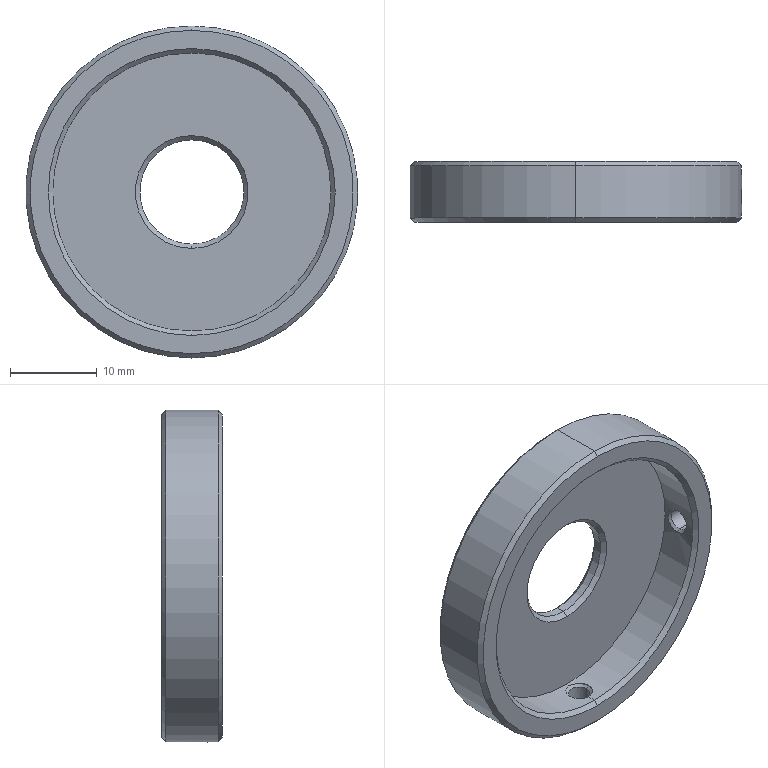Part | SolidWorks | features 3DProfileFeature 1, HoleWzd 1, ICE 1, Revolution 1 | 1 solid | 33 faces | box 38.2 x 7 x 38.2 mm | volume 3692 mm3 | cylinder 16 | cone 14 | plane 3 | commonest cylinder face diameters 3.05 x6 2.5 x4 12 x2 32 x2 38.2 x2
STEP:
#1=CARTESIAN_POINT('',(16.275,3.,-1.25));
#2=VERTEX_POINT('',#1);
#3=CARTESIAN_POINT('',(16.275,3.,1.25));
#4=VERTEX_POINT('',#3);
#5=CARTESIAN_POINT('',(16.275,3.,0.));
#6=DIRECTION('',(-1.,0.,0.));
#7=DIRECTION('',(0.,0.,1.));
#8=AXIS2_PLACEMENT_3D('',#5,#6,#7);
#9=CIRCLE('',#8,1.25);
#10=EDGE_CURVE('',#2,#4,#9,.T.);
#11=ORIENTED_EDGE('',*,*,#10,.F.);
#12=CARTESIAN_POINT('',(16.,3.,-1.525));
#13=VERTEX_POINT('',#12);
#14=CARTESIAN_POINT('',(16.,3.,-1.525));
#15=DIRECTION('',(-0.7071,0.,-0.7071));
#16=VECTOR('',#15,1000.);
#17=LINE('',#14,#16);
#18=EDGE_CURVE('',#2,#13,#17,.T.);
#19=ORIENTED_EDGE('',*,*,#18,.T.);
#20=CARTESIAN_POINT('',(16.,1.475,0.));
#21=VERTEX_POINT('',#20);
#22=CARTESIAN_POINT('',(16.,3.,0.));
#23=DIRECTION('',(-1.,0.,0.));
#24=DIRECTION('',(0.,0.,1.));
#25=AXIS2_PLACEMENT_3D('',#22,#23,#24);
#26=CIRCLE('',#25,1.525);
#27=EDGE_CURVE('',#13,#21,#26,.T.);
#28=ORIENTED_EDGE('',*,*,#27,.T.);
#29=CARTESIAN_POINT('',(16.,3.,1.525));
#30=VERTEX_POINT('',#29);
#31=CARTESIAN_POINT('',(16.,3.,0.));
#32=DIRECTION('',(-1.,0.,0.));
#33=DIRECTION('',(0.,0.,1.));
#34=AXIS2_PLACEMENT_3D('',#31,#32,#33);
#35=CIRCLE('',#34,1.525);
#36=EDGE_CURVE('',#21,#30,#35,.T.);
#37=ORIENTED_EDGE('',*,*,#36,.T.);
#38=CARTESIAN_POINT('',(16.,3.,1.525));
#39=DIRECTION('',(-0.7071,0.,0.7071));
#40=VECTOR('',#39,1000.);
#41=LINE('',#38,#40);
#42=EDGE_CURVE('',#4,#30,#41,.T.);
#43=ORIENTED_EDGE('',*,*,#42,.F.);
#44=EDGE_LOOP('',(#11,#19,#28,#37,#43));
#45=FACE_OUTER_BOUND('',#44,.T.);
#46=CARTESIAN_POINT('',(16.,3.,0.));
#47=DIRECTION('',(-1.,0.,0.));
#48=DIRECTION('',(0.,0.,1.));
#49=AXIS2_PLACEMENT_3D('',#46,#47,#48);
#50=CONICAL_SURFACE('',#49,1.525,0.7854);
#51=ADVANCED_FACE('',(#45),#50,.F.);
#52=CARTESIAN_POINT('',(19.059,3.,1.25));
#53=VERTEX_POINT('',#52);
#54=CARTESIAN_POINT('',(19.059,3.,-1.25));
#55=VERTEX_POINT('',#54);
#56=CARTESIAN_POINT('',(19.059,3.,1.25));
#57=CARTESIAN_POINT('',(19.059,2.835,1.25));
#58=CARTESIAN_POINT('',(19.061,2.673,1.218));
#59=CARTESIAN_POINT('',(19.067,2.446,1.123));
#60=CARTESIAN_POINT('',(19.069,2.374,1.085));
#61=CARTESIAN_POINT('',(19.074,2.238,0.9943));
#62=CARTESIAN_POINT('',(19.077,2.174,0.9415));
#63=CARTESIAN_POINT('',(19.085,2.001,0.7685));
#64=CARTESIAN_POINT('',(19.09,1.908,0.6291));
#65=CARTESIAN_POINT('',(19.098,1.783,0.3284));
#66=CARTESIAN_POINT('',(19.1,1.75,0.1642));
#67=CARTESIAN_POINT('',(19.1,1.75,-0.1661));
#68=CARTESIAN_POINT('',(19.098,1.783,-0.3282));
#69=CARTESIAN_POINT('',(19.09,1.908,-0.6308));
#70=CARTESIAN_POINT('',(19.085,2.001,-0.7694));
#71=CARTESIAN_POINT('',(19.074,2.232,-0.9997));
#72=CARTESIAN_POINT('',(19.069,2.372,-1.093));
#73=CARTESIAN_POINT('',(19.061,2.672,-1.217));
#74=CARTESIAN_POINT('',(19.059,2.837,-1.25));
#75=CARTESIAN_POINT('',(19.059,3.,-1.25));
#76=B_SPLINE_CURVE_WITH_KNOTS('',3,(#56,#57,#58,#59,#60,#61,#62,#63,#64,#65,#66,#67,#68,#69,#70,#71,#72,#73,#74,#75),.UNSPECIFIED.,.F.,.F.,(4,2,2,2,2,2,2,2,2,4),(0.005864,0.006353,0.006597,0.006841,0.00733,0.007818,0.008307,0.008795,0.009284,0.009772),.UNSPECIFIED.);
#77=EDGE_CURVE('',#53,#55,#76,.T.);
#78=ORIENTED_EDGE('',*,*,#77,.T.);
#79=CARTESIAN_POINT('',(16.,3.,-1.25));
#80=DIRECTION('',(-1.,0.,0.));
#81=VECTOR('',#80,1000.);
#82=LINE('',#79,#81);
#83=EDGE_CURVE('',#55,#2,#82,.T.);
#84=ORIENTED_EDGE('',*,*,#83,.T.);
#85=ORIENTED_EDGE('',*,*,#10,.T.);
#86=CARTESIAN_POINT('',(16.,3.,1.25));
#87=DIRECTION('',(-1.,0.,0.));
#88=VECTOR('',#87,1000.);
#89=LINE('',#86,#88);
#90=EDGE_CURVE('',#53,#4,#89,.T.);
#91=ORIENTED_EDGE('',*,*,#90,.F.);
#92=EDGE_LOOP('',(#78,#84,#85,#91));
#93=FACE_OUTER_BOUND('',#92,.T.);
#94=CARTESIAN_POINT('',(16.,3.,0.));
#95=DIRECTION('',(-1.,0.,0.));
#96=DIRECTION('',(0.,0.,1.));
#97=AXIS2_PLACEMENT_3D('',#94,#95,#96);
#98=CYLINDRICAL_SURFACE('',#97,1.25);
#99=ADVANCED_FACE('',(#93),#98,.F.);
#100=CARTESIAN_POINT('',(16.,4.525,0.));
#101=VERTEX_POINT('',#100);
#102=CARTESIAN_POINT('',(16.,3.,0.));
#103=DIRECTION('',(-1.,0.,0.));
#104=DIRECTION('',(0.,0.,1.));
#105=AXIS2_PLACEMENT_3D('',#102,#103,#104);
#106=CIRCLE('',#105,1.525);
#107=EDGE_CURVE('',#30,#101,#106,.T.);
#108=ORIENTED_EDGE('',*,*,#107,.F.);
#109=CARTESIAN_POINT('',(15.927,3.,1.525));
#110=VERTEX_POINT('',#109);
#111=CARTESIAN_POINT('',(16.,3.,1.525));
#112=DIRECTION('',(-1.,0.,0.));
#113=VECTOR('',#112,1000.);
#114=LINE('',#111,#113);
#115=EDGE_CURVE('',#30,#110,#114,.T.);
#116=ORIENTED_EDGE('',*,*,#115,.T.);
#117=CARTESIAN_POINT('',(15.927,3.,1.525));
#118=CARTESIAN_POINT('',(15.927,3.1,1.525));
#119=CARTESIAN_POINT('',(15.928,3.201,1.515));
#120=CARTESIAN_POINT('',(15.932,3.396,1.476));
#121=CARTESIAN_POINT('',(15.934,3.491,1.447));
#122=CARTESIAN_POINT('',(15.941,3.676,1.371));
#123=CARTESIAN_POINT('',(15.945,3.765,1.323));
#124=CARTESIAN_POINT('',(15.954,3.93,1.213));
#125=CARTESIAN_POINT('',(15.959,4.007,1.15));
#126=CARTESIAN_POINT('',(15.968,4.15,1.007));
#127=CARTESIAN_POINT('',(15.973,4.213,0.9301));
#128=CARTESIAN_POINT('',(15.982,4.323,0.765));
#129=CARTESIAN_POINT('',(15.986,4.371,0.6759));
#130=CARTESIAN_POINT('',(15.993,4.447,0.4912));
#131=CARTESIAN_POINT('',(15.995,4.476,0.3961));
#132=CARTESIAN_POINT('',(15.999,4.515,0.2006));
#133=CARTESIAN_POINT('',(16.,4.525,0.09953));
#134=CARTESIAN_POINT('',(16.,4.525,0.));
#135=B_SPLINE_CURVE_WITH_KNOTS('',3,(#117,#118,#119,#120,#121,#122,#123,#124,#125,#126,#127,#128,#129,#130,#131,#132,#133,#134),.UNSPECIFIED.,.F.,.F.,(4,2,2,2,2,2,2,2,4),(0.002386,0.002684,0.002982,0.00328,0.003578,0.003876,0.004174,0.004472,0.004771),.UNSPECIFIED.);
#136=EDGE_CURVE('',#110,#101,#135,.T.);
#137=ORIENTED_EDGE('',*,*,#136,.T.);
#138=EDGE_LOOP('',(#108,#116,#137));
#139=FACE_OUTER_BOUND('',#138,.T.);
#140=CARTESIAN_POINT('',(16.,3.,0.));
#141=DIRECTION('',(-1.,0.,0.));
#142=DIRECTION('',(0.,0.,1.));
#143=AXIS2_PLACEMENT_3D('',#140,#141,#142);
#144=CYLINDRICAL_SURFACE('',#143,1.525);
#145=ADVANCED_FACE('',(#139),#144,.F.);
#146=CARTESIAN_POINT('',(-1.25,3.,-16.275));
#147=VERTEX_POINT('',#146);
#148=CARTESIAN_POINT('',(1.25,3.,-16.275));
#149=VERTEX_POINT('',#148);
#150=CARTESIAN_POINT('',(0.,3.,-16.275));
#151=DIRECTION('',(0.,0.,1.));
#152=DIRECTION('',(1.,0.,0.));
#153=AXIS2_PLACEMENT_3D('',#150,#151,#152);
#154=CIRCLE('',#153,1.25);
#155=EDGE_CURVE('',#147,#149,#154,.T.);
#156=ORIENTED_EDGE('',*,*,#155,.F.);
#157=CARTESIAN_POINT('',(-1.525,3.,-16.));
#158=VERTEX_POINT('',#157);
#159=CARTESIAN_POINT('',(-1.525,3.,-16.));
#160=DIRECTION('',(-0.7071,0.,0.7071));
#161=VECTOR('',#160,1000.);
#162=LINE('',#159,#161);
#163=EDGE_CURVE('',#147,#158,#162,.T.);
#164=ORIENTED_EDGE('',*,*,#163,.T.);
#165=CARTESIAN_POINT('',(0.,1.475,-16.));
#166=VERTEX_POINT('',#165);
#167=CARTESIAN_POINT('',(0.,3.,-16.));
#168=DIRECTION('',(0.,0.,1.));
#169=DIRECTION('',(1.,0.,0.));
#170=AXIS2_PLACEMENT_3D('',#167,#168,#169);
#171=CIRCLE('',#170,1.525);
#172=EDGE_CURVE('',#158,#166,#171,.T.);
#173=ORIENTED_EDGE('',*,*,#172,.T.);
#174=CARTESIAN_POINT('',(1.525,3.,-16.));
#175=VERTEX_POINT('',#174);
#176=CARTESIAN_POINT('',(0.,3.,-16.));
#177=DIRECTION('',(0.,0.,1.));
#178=DIRECTION('',(1.,0.,0.));
#179=AXIS2_PLACEMENT_3D('',#176,#177,#178);
#180=CIRCLE('',#179,1.525);
#181=EDGE_CURVE('',#166,#175,#180,.T.);
#182=ORIENTED_EDGE('',*,*,#181,.T.);
#183=CARTESIAN_POINT('',(1.525,3.,-16.));
#184=DIRECTION('',(0.7071,0.,0.7071));
#185=VECTOR('',#184,1000.);
#186=LINE('',#183,#185);
#187=EDGE_CURVE('',#149,#175,#186,.T.);
#188=ORIENTED_EDGE('',*,*,#187,.F.);
#189=EDGE_LOOP('',(#156,#164,#173,#182,#188));
#190=FACE_OUTER_BOUND('',#189,.T.);
#191=CARTESIAN_POINT('',(0.,3.,-16.));
#192=DIRECTION('',(0.,0.,1.));
#193=DIRECTION('',(1.,0.,0.));
#194=AXIS2_PLACEMENT_3D('',#191,#192,#193);
#195=CONICAL_SURFACE('',#194,1.525,0.7854);
#196=ADVANCED_FACE('',(#190),#195,.F.);
#197=CARTESIAN_POINT('',(0.,1.75,-19.1));
#198=VERTEX_POINT('',#197);
#199=CARTESIAN_POINT('',(-1.25,3.,-19.059));
#200=VERTEX_POINT('',#199);
#201=CARTESIAN_POINT('',(0.,1.75,-19.1));
#202=CARTESIAN_POINT('',(-0.1632,1.75,-19.1));
#203=CARTESIAN_POINT('',(-0.3278,1.783,-19.098));
#204=CARTESIAN_POINT('',(-0.6288,1.907,-19.09));
#205=CARTESIAN_POINT('',(-0.7683,2.001,-19.085));
#206=CARTESIAN_POINT('',(-0.9989,2.231,-19.074));
#207=CARTESIAN_POINT('',(-1.092,2.37,-19.069));
#208=CARTESIAN_POINT('',(-1.217,2.673,-19.061));
#209=CARTESIAN_POINT('',(-1.25,2.835,-19.059));
#210=CARTESIAN_POINT('',(-1.25,3.,-19.059));
#211=B_SPLINE_CURVE_WITH_KNOTS('',3,(#201,#202,#203,#204,#205,#206,#207,#208,#209,#210),.UNSPECIFIED.,.F.,.F.,(4,2,2,2,4),(0.003909,0.004398,0.004887,0.005375,0.005864),.UNSPECIFIED.);
#212=EDGE_CURVE('',#198,#200,#211,.T.);
#213=ORIENTED_EDGE('',*,*,#212,.T.);
#214=CARTESIAN_POINT('',(-1.25,3.,-16.));
#215=DIRECTION('',(0.,0.,1.));
#216=VECTOR('',#215,1000.);
#217=LINE('',#214,#216);
#218=EDGE_CURVE('',#200,#147,#217,.T.);
#219=ORIENTED_EDGE('',*,*,#218,.T.);
#220=ORIENTED_EDGE('',*,*,#155,.T.);
#221=CARTESIAN_POINT('',(1.25,3.,-19.059));
#222=VERTEX_POINT('',#221);
#223=CARTESIAN_POINT('',(1.25,3.,-16.));
#224=DIRECTION('',(0.,0.,1.));
#225=VECTOR('',#224,1000.);
#226=LINE('',#223,#225);
#227=EDGE_CURVE('',#222,#149,#226,.T.);
#228=ORIENTED_EDGE('',*,*,#227,.F.);
#229=CARTESIAN_POINT('',(1.25,3.,-19.059));
#230=CARTESIAN_POINT('',(1.25,2.837,-19.059));
#231=CARTESIAN_POINT('',(1.218,2.673,-19.061));
#232=CARTESIAN_POINT('',(1.092,2.37,-19.069));
#233=CARTESIAN_POINT('',(1.001,2.233,-19.074));
#234=CARTESIAN_POINT('',(0.7672,1.999,-19.085));
#235=CARTESIAN_POINT('',(0.6297,1.908,-19.09));
#236=CARTESIAN_POINT('',(0.4025,1.814,-19.096));
#237=CARTESIAN_POINT('',(0.3246,1.79,-19.097));
#238=CARTESIAN_POINT('',(0.1644,1.758,-19.099));
#239=CARTESIAN_POINT('',(0.08157,1.75,-19.1));
#240=CARTESIAN_POINT('',(0.,1.75,-19.1));
#241=B_SPLINE_CURVE_WITH_KNOTS('',3,(#229,#230,#231,#232,#233,#234,#235,#236,#237,#238,#239,#240),.UNSPECIFIED.,.F.,.F.,(4,2,2,2,2,4),(0.001955,0.002444,0.002932,0.003421,0.003665,0.003909),.UNSPECIFIED.);
#242=EDGE_CURVE('',#222,#198,#241,.T.);
#243=ORIENTED_EDGE('',*,*,#242,.T.);
#244=EDGE_LOOP('',(#213,#219,#220,#228,#243));
#245=FACE_OUTER_BOUND('',#244,.T.);
#246=CARTESIAN_POINT('',(0.,3.,-16.));
#247=DIRECTION('',(0.,0.,1.));
#248=DIRECTION('',(1.,0.,0.));
#249=AXIS2_PLACEMENT_3D('',#246,#247,#248);
#250=CYLINDRICAL_SURFACE('',#249,1.25);
#251=ADVANCED_FACE('',(#245),#250,.F.);
#252=CARTESIAN_POINT('',(0.,4.525,-16.));
#253=VERTEX_POINT('',#252);
#254=CARTESIAN_POINT('',(0.,3.,-16.));
#255=DIRECTION('',(0.,0.,1.));
#256=DIRECTION('',(1.,0.,0.));
#257=AXIS2_PLACEMENT_3D('',#254,#255,#256);
#258=CIRCLE('',#257,1.525);
#259=EDGE_CURVE('',#175,#253,#258,.T.);
#260=ORIENTED_EDGE('',*,*,#259,.F.);
#261=CARTESIAN_POINT('',(1.525,3.,-15.927));
#262=VERTEX_POINT('',#261);
#263=CARTESIAN_POINT('',(1.525,3.,-16.));
#264=DIRECTION('',(0.,0.,1.));
#265=VECTOR('',#264,1000.);
#266=LINE('',#263,#265);
#267=EDGE_CURVE('',#175,#262,#266,.T.);
#268=ORIENTED_EDGE('',*,*,#267,.T.);
#269=CARTESIAN_POINT('',(1.525,3.,-15.927));
#270=CARTESIAN_POINT('',(1.525,3.201,-15.927));
#271=CARTESIAN_POINT('',(1.485,3.399,-15.931));
#272=CARTESIAN_POINT('',(1.371,3.676,-15.941));
#273=CARTESIAN_POINT('',(1.324,3.764,-15.945));
#274=CARTESIAN_POINT('',(1.213,3.929,-15.954));
#275=CARTESIAN_POINT('',(1.149,4.008,-15.959));
#276=CARTESIAN_POINT('',(0.9382,4.219,-15.973));
#277=CARTESIAN_POINT('',(0.7683,4.332,-15.983));
#278=CARTESIAN_POINT('',(0.4017,4.484,-15.996));
#279=CARTESIAN_POINT('',(0.2015,4.525,-16.));
#280=CARTESIAN_POINT('',(0.,4.525,-16.));
#281=B_SPLINE_CURVE_WITH_KNOTS('',3,(#269,#270,#271,#272,#273,#274,#275,#276,#277,#278,#279,#280),.UNSPECIFIED.,.F.,.F.,(4,2,2,2,2,4),(0.007156,0.007752,0.00805,0.008348,0.008944,0.00954),.UNSPECIFIED.);
#282=EDGE_CURVE('',#262,#253,#281,.T.);
#283=ORIENTED_EDGE('',*,*,#282,.T.);
#284=EDGE_LOOP('',(#260,#268,#283));
#285=FACE_OUTER_BOUND('',#284,.T.);
#286=CARTESIAN_POINT('',(0.,3.,-16.));
#287=DIRECTION('',(0.,0.,1.));
#288=DIRECTION('',(1.,0.,0.));
#289=AXIS2_PLACEMENT_3D('',#286,#287,#288);
#290=CYLINDRICAL_SURFACE('',#289,1.525);
#291=ADVANCED_FACE('',(#285),#290,.F.);
#292=CARTESIAN_POINT('',(0.,7.,-18.6));
#293=VERTEX_POINT('',#292);
#294=CARTESIAN_POINT('',(0.,7.,18.6));
#295=VERTEX_POINT('',#294);
#296=CARTESIAN_POINT('',(0.,7.,0.));
#297=DIRECTION('',(0.,-1.,0.));
#298=DIRECTION('',(0.,0.,-1.));
#299=AXIS2_PLACEMENT_3D('',#296,#297,#298);
#300=CIRCLE('',#299,18.6);
#301=EDGE_CURVE('',#293,#295,#300,.T.);
#302=ORIENTED_EDGE('',*,*,#301,.T.);
#303=CARTESIAN_POINT('',(0.,6.5,19.1));
#304=VERTEX_POINT('',#303);
#305=CARTESIAN_POINT('',(0.,6.5,19.1));
#306=DIRECTION('',(0.,-0.7071,0.7071));
#307=VECTOR('',#306,1000.);
#308=LINE('',#305,#307);
#309=EDGE_CURVE('',#295,#304,#308,.T.);
#310=ORIENTED_EDGE('',*,*,#309,.T.);
#311=CARTESIAN_POINT('',(0.,6.5,-19.1));
#312=VERTEX_POINT('',#311);
#313=CARTESIAN_POINT('',(0.,6.5,0.));
#314=DIRECTION('',(0.,-1.,0.));
#315=DIRECTION('',(0.,0.,-1.));
#316=AXIS2_PLACEMENT_3D('',#313,#314,#315);
#317=CIRCLE('',#316,19.1);
#318=EDGE_CURVE('',#312,#304,#317,.T.);
#319=ORIENTED_EDGE('',*,*,#318,.F.);
#320=CARTESIAN_POINT('',(0.,6.5,-19.1));
#321=DIRECTION('',(0.,-0.7071,-0.7071));
#322=VECTOR('',#321,1000.);
#323=LINE('',#320,#322);
#324=EDGE_CURVE('',#293,#312,#323,.T.);
#325=ORIENTED_EDGE('',*,*,#324,.F.);
#326=EDGE_LOOP('',(#302,#310,#319,#325));
#327=FACE_OUTER_BOUND('',#326,.T.);
#328=CARTESIAN_POINT('',(0.,6.5,0.));
#329=DIRECTION('',(0.,-1.,0.));
#330=DIRECTION('',(0.,0.,-1.));
#331=AXIS2_PLACEMENT_3D('',#328,#329,#330);
#332=CONICAL_SURFACE('',#331,19.1,0.7854);
#333=ADVANCED_FACE('',(#327),#332,.T.);
#334=ORIENTED_EDGE('',*,*,#77,.F.);
#335=CARTESIAN_POINT('',(19.059,3.,-1.25));
#336=CARTESIAN_POINT('',(19.059,3.163,-1.25));
#337=CARTESIAN_POINT('',(19.061,3.327,-1.218));
#338=CARTESIAN_POINT('',(19.069,3.63,-1.092));
#339=CARTESIAN_POINT('',(19.074,3.767,-1.));
#340=CARTESIAN_POINT('',(19.085,4.001,-0.767));
#341=CARTESIAN_POINT('',(19.09,4.092,-0.6294));
#342=CARTESIAN_POINT('',(19.096,4.186,-0.4021));
#343=CARTESIAN_POINT('',(19.097,4.21,-0.3242));
#344=CARTESIAN_POINT('',(19.099,4.242,-0.164));
#345=CARTESIAN_POINT('',(19.1,4.25,-0.08109));
#346=CARTESIAN_POINT('',(19.1,4.25,0.1637));
#347=CARTESIAN_POINT('',(19.098,4.217,0.3282));
#348=CARTESIAN_POINT('',(19.09,4.092,0.6291));
#349=CARTESIAN_POINT('',(19.085,3.999,0.7685));
#350=CARTESIAN_POINT('',(19.074,3.769,0.9991));
#351=CARTESIAN_POINT('',(19.069,3.63,1.092));
#352=CARTESIAN_POINT('',(19.061,3.327,1.217));
#353=CARTESIAN_POINT('',(19.059,3.165,1.25));
#354=CARTESIAN_POINT('',(19.059,3.,1.25));
#355=B_SPLINE_CURVE_WITH_KNOTS('',3,(#335,#336,#337,#338,#339,#340,#341,#342,#343,#344,#345,#346,#347,#348,#349,#350,#351,#352,#353,#354),.UNSPECIFIED.,.F.,.F.,(4,2,2,2,2,2,2,2,2,4),(0.001955,0.002444,0.002932,0.003421,0.003665,0.00391,0.004398,0.004887,0.005376,0.005864),.UNSPECIFIED.);
#356=EDGE_CURVE('',#55,#53,#355,.T.);
#357=ORIENTED_EDGE('',*,*,#356,.F.);
#358=EDGE_LOOP('',(#334,#357));
#359=FACE_BOUND('',#358,.T.);
#360=ORIENTED_EDGE('',*,*,#318,.T.);
#361=CARTESIAN_POINT('',(0.,0.5,19.1));
#362=VERTEX_POINT('',#361);
#363=CARTESIAN_POINT('',(0.,0.,19.1));
#364=DIRECTION('',(0.,-1.,0.));
#365=VECTOR('',#364,1000.);
#366=LINE('',#363,#365);
#367=EDGE_CURVE('',#304,#362,#366,.T.);
#368=ORIENTED_EDGE('',*,*,#367,.T.);
#369=CARTESIAN_POINT('',(0.,0.5,-19.1));
#370=VERTEX_POINT('',#369);
#371=CARTESIAN_POINT('',(0.,0.5,0.));
#372=DIRECTION('',(0.,-1.,0.));
#373=DIRECTION('',(0.,0.,-1.));
#374=AXIS2_PLACEMENT_3D('',#371,#372,#373);
#375=CIRCLE('',#374,19.1);
#376=EDGE_CURVE('',#370,#362,#375,.T.);
#377=ORIENTED_EDGE('',*,*,#376,.F.);
#378=CARTESIAN_POINT('',(0.,0.,-19.1));
#379=DIRECTION('',(0.,-1.,0.));
#380=VECTOR('',#379,1000.);
#381=LINE('',#378,#380);
#382=EDGE_CURVE('',#198,#370,#381,.T.);
#383=ORIENTED_EDGE('',*,*,#382,.F.);
#384=ORIENTED_EDGE('',*,*,#242,.F.);
#385=CARTESIAN_POINT('',(0.,4.25,-19.1));
#386=VERTEX_POINT('',#385);
#387=CARTESIAN_POINT('',(0.,4.25,-19.1));
#388=CARTESIAN_POINT('',(0.1653,4.25,-19.1));
#389=CARTESIAN_POINT('',(0.3274,4.217,-19.098));
#390=CARTESIAN_POINT('',(0.6303,4.092,-19.09));
#391=CARTESIAN_POINT('',(0.7689,3.999,-19.085));
#392=CARTESIAN_POINT('',(0.9995,3.768,-19.074));
#393=CARTESIAN_POINT('',(1.093,3.629,-19.069));
#394=CARTESIAN_POINT('',(1.217,3.328,-19.061));
#395=CARTESIAN_POINT('',(1.25,3.163,-19.059));
#396=CARTESIAN_POINT('',(1.25,3.,-19.059));
#397=B_SPLINE_CURVE_WITH_KNOTS('',3,(#387,#388,#389,#390,#391,#392,#393,#394,#395,#396),.UNSPECIFIED.,.F.,.F.,(4,2,2,2,4),(0.,0.0004888,0.0009775,0.001466,0.001955),.UNSPECIFIED.);
#398=EDGE_CURVE('',#386,#222,#397,.T.);
#399=ORIENTED_EDGE('',*,*,#398,.F.);
#400=CARTESIAN_POINT('',(0.,0.,-19.1));
#401=DIRECTION('',(0.,-1.,0.));
#402=VECTOR('',#401,1000.);
#403=LINE('',#400,#402);
#404=EDGE_CURVE('',#312,#386,#403,.T.);
#405=ORIENTED_EDGE('',*,*,#404,.F.);
#406=EDGE_LOOP('',(#360,#368,#377,#383,#384,#399,#405));
#407=FACE_OUTER_BOUND('',#406,.T.);
#408=CARTESIAN_POINT('',(0.,0.,0.));
#409=DIRECTION('',(0.,-1.,0.));
#410=DIRECTION('',(0.,0.,-1.));
#411=AXIS2_PLACEMENT_3D('',#408,#409,#410);
#412=CYLINDRICAL_SURFACE('',#411,19.1);
#413=ADVANCED_FACE('',(#359,#407),#412,.T.);
#414=CARTESIAN_POINT('',(0.,0.,-18.6));
#415=VERTEX_POINT('',#414);
#416=CARTESIAN_POINT('',(0.,0.,18.6));
#417=VERTEX_POINT('',#416);
#418=CARTESIAN_POINT('',(0.,0.,0.));
#419=DIRECTION('',(0.,-1.,0.));
#420=DIRECTION('',(0.,0.,-1.));
#421=AXIS2_PLACEMENT_3D('',#418,#419,#420);
#422=CIRCLE('',#421,18.6);
#423=EDGE_CURVE('',#415,#417,#422,.T.);
#424=ORIENTED_EDGE('',*,*,#423,.F.);
#425=CARTESIAN_POINT('',(0.,0.,-18.6));
#426=DIRECTION('',(0.,0.7071,-0.7071));
#427=VECTOR('',#426,1000.);
#428=LINE('',#425,#427);
#429=EDGE_CURVE('',#415,#370,#428,.T.);
#430=ORIENTED_EDGE('',*,*,#429,.T.);
#431=ORIENTED_EDGE('',*,*,#376,.T.);
#432=CARTESIAN_POINT('',(0.,0.,18.6));
#433=DIRECTION('',(0.,0.7071,0.7071));
#434=VECTOR('',#433,1000.);
#435=LINE('',#432,#434);
#436=EDGE_CURVE('',#417,#362,#435,.T.);
#437=ORIENTED_EDGE('',*,*,#436,.F.);
#438=EDGE_LOOP('',(#424,#430,#431,#437));
#439=FACE_OUTER_BOUND('',#438,.T.);
#440=CARTESIAN_POINT('',(0.,0.,0.));
#441=DIRECTION('',(0.,1.,0.));
#442=DIRECTION('',(0.,0.,1.));
#443=AXIS2_PLACEMENT_3D('',#440,#441,#442);
#444=CONICAL_SURFACE('',#443,18.6,0.7854);
#445=ADVANCED_FACE('',(#439),#444,.T.);
#446=CARTESIAN_POINT('',(0.,0.5,16.));
#447=VERTEX_POINT('',#446);
#448=CARTESIAN_POINT('',(0.,0.5,-16.));
#449=VERTEX_POINT('',#448);
#450=CARTESIAN_POINT('',(0.,0.5,0.));
#451=DIRECTION('',(0.,-1.,0.));
#452=DIRECTION('',(0.,0.,-1.));
#453=AXIS2_PLACEMENT_3D('',#450,#451,#452);
#454=CIRCLE('',#453,16.);
#455=EDGE_CURVE('',#447,#449,#454,.T.);
#456=ORIENTED_EDGE('',*,*,#455,.F.);
#457=CARTESIAN_POINT('',(0.,0.,16.5));
#458=VERTEX_POINT('',#457);
#459=CARTESIAN_POINT('',(0.,0.5,16.));
#460=DIRECTION('',(0.,-0.7071,0.7071));
#461=VECTOR('',#460,1000.);
#462=LINE('',#459,#461);
#463=EDGE_CURVE('',#447,#458,#462,.T.);
#464=ORIENTED_EDGE('',*,*,#463,.T.);
#465=CARTESIAN_POINT('',(0.,0.,-16.5));
#466=VERTEX_POINT('',#465);
#467=CARTESIAN_POINT('',(0.,0.,0.));
#468=DIRECTION('',(0.,-1.,0.));
#469=DIRECTION('',(0.,0.,-1.));
#470=AXIS2_PLACEMENT_3D('',#467,#468,#469);
#471=CIRCLE('',#470,16.5);
#472=EDGE_CURVE('',#458,#466,#471,.T.);
#473=ORIENTED_EDGE('',*,*,#472,.T.);
#474=CARTESIAN_POINT('',(0.,0.5,-16.));
#475=DIRECTION('',(0.,-0.7071,-0.7071));
#476=VECTOR('',#475,1000.);
#477=LINE('',#474,#476);
#478=EDGE_CURVE('',#449,#466,#477,.T.);
#479=ORIENTED_EDGE('',*,*,#478,.F.);
#480=EDGE_LOOP('',(#456,#464,#473,#479));
#481=FACE_OUTER_BOUND('',#480,.T.);
#482=CARTESIAN_POINT('',(0.,0.5,0.));
#483=DIRECTION('',(0.,-1.,0.));
#484=DIRECTION('',(0.,0.,-1.));
#485=AXIS2_PLACEMENT_3D('',#482,#483,#484);
#486=CONICAL_SURFACE('',#485,16.,0.7854);
#487=ADVANCED_FACE('',(#481),#486,.F.);
#488=CARTESIAN_POINT('',(0.,5.,16.));
#489=VERTEX_POINT('',#488);
#490=CARTESIAN_POINT('',(0.,5.,-16.));
#491=VERTEX_POINT('',#490);
#492=CARTESIAN_POINT('',(0.,5.,0.));
#493=DIRECTION('',(0.,-1.,0.));
#494=DIRECTION('',(0.,0.,-1.));
#495=AXIS2_PLACEMENT_3D('',#492,#493,#494);
#496=CIRCLE('',#495,16.);
#497=EDGE_CURVE('',#489,#491,#496,.T.);
#498=ORIENTED_EDGE('',*,*,#497,.F.);
#499=CARTESIAN_POINT('',(0.,0.,16.));
#500=DIRECTION('',(0.,-1.,0.));
#501=VECTOR('',#500,1000.);
#502=LINE('',#499,#501);
#503=EDGE_CURVE('',#489,#447,#502,.T.);
#504=ORIENTED_EDGE('',*,*,#503,.T.);
#505=ORIENTED_EDGE('',*,*,#455,.T.);
#506=CARTESIAN_POINT('',(0.,0.,-16.));
#507=DIRECTION('',(0.,-1.,0.));
#508=VECTOR('',#507,1000.);
#509=LINE('',#506,#508);
#510=EDGE_CURVE('',#166,#449,#509,.T.);
#511=ORIENTED_EDGE('',*,*,#510,.F.);
#512=CARTESIAN_POINT('',(0.,4.525,-16.));
#513=CARTESIAN_POINT('',(-0.1008,4.525,-16.));
#514=CARTESIAN_POINT('',(-0.1999,4.515,-15.999));
#515=CARTESIAN_POINT('',(-0.3949,4.476,-15.995));
#516=CARTESIAN_POINT('',(-0.4918,4.447,-15.993));
#517=CARTESIAN_POINT('',(-0.6765,4.37,-15.986));
#518=CARTESIAN_POINT('',(-0.7641,4.324,-15.982));
#519=CARTESIAN_POINT('',(-0.9298,4.213,-15.973));
#520=CARTESIAN_POINT('',(-1.008,4.148,-15.968));
#521=CARTESIAN_POINT('',(-1.219,3.937,-15.954));
#522=CARTESIAN_POINT('',(-1.333,3.767,-15.945));
#523=CARTESIAN_POINT('',(-1.485,3.4,-15.931));
#524=CARTESIAN_POINT('',(-1.525,3.2,-15.927));
#525=CARTESIAN_POINT('',(-1.525,2.901,-15.927));
#526=CARTESIAN_POINT('',(-1.515,2.8,-15.928));
#527=CARTESIAN_POINT('',(-1.476,2.604,-15.932));
#528=CARTESIAN_POINT('',(-1.447,2.509,-15.934));
#529=CARTESIAN_POINT('',(-1.371,2.324,-15.941));
#530=CARTESIAN_POINT('',(-1.323,2.235,-15.945));
#531=CARTESIAN_POINT('',(-1.213,2.07,-15.954));
#532=CARTESIAN_POINT('',(-1.15,1.993,-15.959));
#533=CARTESIAN_POINT('',(-1.007,1.851,-15.968));
#534=CARTESIAN_POINT('',(-0.9303,1.788,-15.973));
#535=CARTESIAN_POINT('',(-0.7652,1.677,-15.982));
#536=CARTESIAN_POINT('',(-0.676,1.629,-15.986));
#537=CARTESIAN_POINT('',(-0.4913,1.553,-15.993));
#538=CARTESIAN_POINT('',(-0.3962,1.524,-15.995));
#539=CARTESIAN_POINT('',(-0.2007,1.485,-15.999));
#540=CARTESIAN_POINT('',(-0.09956,1.475,-16.));
#541=CARTESIAN_POINT('',(0.,1.475,-16.));
#542=B_SPLINE_CURVE_WITH_KNOTS('',3,(#512,#513,#514,#515,#516,#517,#518,#519,#520,#521,#522,#523,#524,#525,#526,#527,#528,#529,#530,#531,#532,#533,#534,#535,#536,#537,#538,#539,#540,#541),.UNSPECIFIED.,.F.,.F.,(4,2,2,2,2,2,2,2,2,2,2,2,2,2,4),(0.,0.0002982,0.0005963,0.0008945,0.001193,0.001789,0.002385,0.002683,0.002982,0.00328,0.003578,0.003876,0.004174,0.004472,0.004771),.UNSPECIFIED.);
#543=EDGE_CURVE('',#253,#166,#542,.T.);
#544=ORIENTED_EDGE('',*,*,#543,.F.);
#545=CARTESIAN_POINT('',(0.,0.,-16.));
#546=DIRECTION('',(0.,-1.,0.));
#547=VECTOR('',#546,1000.);
#548=LINE('',#545,#547);
#549=EDGE_CURVE('',#491,#253,#548,.T.);
#550=ORIENTED_EDGE('',*,*,#549,.F.);
#551=EDGE_LOOP('',(#498,#504,#505,#511,#544,#550));
#552=FACE_OUTER_BOUND('',#551,.T.);
#553=CARTESIAN_POINT('',(0.,0.,0.));
#554=DIRECTION('',(0.,-1.,0.));
#555=DIRECTION('',(0.,0.,-1.));
#556=AXIS2_PLACEMENT_3D('',#553,#554,#555);
#557=CYLINDRICAL_SURFACE('',#556,16.);
#558=ADVANCED_FACE('',(#552),#557,.F.);
#559=CARTESIAN_POINT('',(0.,5.5,6.));
#560=VERTEX_POINT('',#559);
#561=CARTESIAN_POINT('',(0.,5.5,-6.));
#562=VERTEX_POINT('',#561);
#563=CARTESIAN_POINT('',(0.,5.5,0.));
#564=DIRECTION('',(0.,-1.,0.));
#565=DIRECTION('',(0.,0.,-1.));
#566=AXIS2_PLACEMENT_3D('',#563,#564,#565);
#567=CIRCLE('',#566,6.);
#568=EDGE_CURVE('',#560,#562,#567,.T.);
#569=ORIENTED_EDGE('',*,*,#568,.F.);
#570=CARTESIAN_POINT('',(0.,5.,6.5));
#571=VERTEX_POINT('',#570);
#572=CARTESIAN_POINT('',(0.,5.5,6.));
#573=DIRECTION('',(0.,-0.7071,0.7071));
#574=VECTOR('',#573,1000.);
#575=LINE('',#572,#574);
#576=EDGE_CURVE('',#560,#571,#575,.T.);
#577=ORIENTED_EDGE('',*,*,#576,.T.);
#578=CARTESIAN_POINT('',(0.,5.,-6.5));
#579=VERTEX_POINT('',#578);
#580=CARTESIAN_POINT('',(0.,5.,0.));
#581=DIRECTION('',(0.,-1.,0.));
#582=DIRECTION('',(0.,0.,-1.));
#583=AXIS2_PLACEMENT_3D('',#580,#581,#582);
#584=CIRCLE('',#583,6.5);
#585=EDGE_CURVE('',#571,#579,#584,.T.);
#586=ORIENTED_EDGE('',*,*,#585,.T.);
#587=CARTESIAN_POINT('',(0.,5.5,-6.));
#588=DIRECTION('',(0.,-0.7071,-0.7071));
#589=VECTOR('',#588,1000.);
#590=LINE('',#587,#589);
#591=EDGE_CURVE('',#562,#579,#590,.T.);
#592=ORIENTED_EDGE('',*,*,#591,.F.);
#593=EDGE_LOOP('',(#569,#577,#586,#592));
#594=FACE_OUTER_BOUND('',#593,.T.);
#595=CARTESIAN_POINT('',(0.,5.5,0.));
#596=DIRECTION('',(0.,-1.,0.));
#597=DIRECTION('',(0.,0.,-1.));
#598=AXIS2_PLACEMENT_3D('',#595,#596,#597);
#599=CONICAL_SURFACE('',#598,6.,0.7854);
#600=ADVANCED_FACE('',(#594),#599,.F.);
#601=CARTESIAN_POINT('',(0.,6.5,6.));
#602=VERTEX_POINT('',#601);
#603=CARTESIAN_POINT('',(0.,6.5,-6.));
#604=VERTEX_POINT('',#603);
#605=CARTESIAN_POINT('',(0.,6.5,0.));
#606=DIRECTION('',(0.,-1.,0.));
#607=DIRECTION('',(0.,0.,-1.));
#608=AXIS2_PLACEMENT_3D('',#605,#606,#607);
#609=CIRCLE('',#608,6.);
#610=EDGE_CURVE('',#602,#604,#609,.T.);
#611=ORIENTED_EDGE('',*,*,#610,.F.);
#612=CARTESIAN_POINT('',(0.,0.,6.));
#613=DIRECTION('',(0.,-1.,0.));
#614=VECTOR('',#613,1000.);
#615=LINE('',#612,#614);
#616=EDGE_CURVE('',#602,#560,#615,.T.);
#617=ORIENTED_EDGE('',*,*,#616,.T.);
#618=ORIENTED_EDGE('',*,*,#568,.T.);
#619=CARTESIAN_POINT('',(0.,0.,-6.));
#620=DIRECTION('',(0.,-1.,0.));
#621=VECTOR('',#620,1000.);
#622=LINE('',#619,#621);
#623=EDGE_CURVE('',#604,#562,#622,.T.);
#624=ORIENTED_EDGE('',*,*,#623,.F.);
#625=EDGE_LOOP('',(#611,#617,#618,#624));
#626=FACE_OUTER_BOUND('',#625,.T.);
#627=CARTESIAN_POINT('',(0.,0.,0.));
#628=DIRECTION('',(0.,-1.,0.));
#629=DIRECTION('',(0.,0.,-1.));
#630=AXIS2_PLACEMENT_3D('',#627,#628,#629);
#631=CYLINDRICAL_SURFACE('',#630,6.);
#632=ADVANCED_FACE('',(#626),#631,.F.);
#633=ORIENTED_EDGE('',*,*,#610,.T.);
#634=CARTESIAN_POINT('',(0.,7.,-6.5));
#635=VERTEX_POINT('',#634);
#636=CARTESIAN_POINT('',(0.,7.,-6.5));
#637=DIRECTION('',(0.,0.7071,-0.7071));
#638=VECTOR('',#637,1000.);
#639=LINE('',#636,#638);
#640=EDGE_CURVE('',#604,#635,#639,.T.);
#641=ORIENTED_EDGE('',*,*,#640,.T.);
#642=CARTESIAN_POINT('',(0.,7.,6.5));
#643=VERTEX_POINT('',#642);
#644=CARTESIAN_POINT('',(0.,7.,0.));
#645=DIRECTION('',(0.,-1.,0.));
#646=DIRECTION('',(0.,0.,-1.));
#647=AXIS2_PLACEMENT_3D('',#644,#645,#646);
#648=CIRCLE('',#647,6.5);
#649=EDGE_CURVE('',#643,#635,#648,.T.);
#650=ORIENTED_EDGE('',*,*,#649,.F.);
#651=CARTESIAN_POINT('',(0.,7.,6.5));
#652=DIRECTION('',(0.,0.7071,0.7071));
#653=VECTOR('',#652,1000.);
#654=LINE('',#651,#653);
#655=EDGE_CURVE('',#602,#643,#654,.T.);
#656=ORIENTED_EDGE('',*,*,#655,.F.);
#657=EDGE_LOOP('',(#633,#641,#650,#656));
#658=FACE_OUTER_BOUND('',#657,.T.);
#659=CARTESIAN_POINT('',(0.,7.,0.));
#660=DIRECTION('',(0.,1.,0.));
#661=DIRECTION('',(0.,0.,1.));
#662=AXIS2_PLACEMENT_3D('',#659,#660,#661);
#663=CONICAL_SURFACE('',#662,6.5,0.7854);
#664=ADVANCED_FACE('',(#658),#663,.F.);
#665=ORIENTED_EDGE('',*,*,#640,.F.);
#666=CARTESIAN_POINT('',(0.,6.5,0.));
#667=DIRECTION('',(0.,-1.,0.));
#668=DIRECTION('',(0.,0.,-1.));
#669=AXIS2_PLACEMENT_3D('',#666,#667,#668);
#670=CIRCLE('',#669,6.);
#671=EDGE_CURVE('',#604,#602,#670,.T.);
#672=ORIENTED_EDGE('',*,*,#671,.T.);
#673=ORIENTED_EDGE('',*,*,#655,.T.);
#674=CARTESIAN_POINT('',(0.,7.,0.));
#675=DIRECTION('',(0.,-1.,0.));
#676=DIRECTION('',(0.,0.,-1.));
#677=AXIS2_PLACEMENT_3D('',#674,#675,#676);
#678=CIRCLE('',#677,6.5);
#679=EDGE_CURVE('',#635,#643,#678,.T.);
#680=ORIENTED_EDGE('',*,*,#679,.F.);
#681=EDGE_LOOP('',(#665,#672,#673,#680));
#682=FACE_OUTER_BOUND('',#681,.T.);
#683=CARTESIAN_POINT('',(0.,7.,0.));
#684=DIRECTION('',(0.,1.,0.));
#685=DIRECTION('',(0.,0.,1.));
#686=AXIS2_PLACEMENT_3D('',#683,#684,#685);
#687=CONICAL_SURFACE('',#686,6.5,0.7854);
#688=ADVANCED_FACE('',(#682),#687,.F.);
#689=ORIENTED_EDGE('',*,*,#616,.F.);
#690=ORIENTED_EDGE('',*,*,#671,.F.);
#691=ORIENTED_EDGE('',*,*,#623,.T.);
#692=CARTESIAN_POINT('',(0.,5.5,0.));
#693=DIRECTION('',(0.,-1.,0.));
#694=DIRECTION('',(0.,0.,-1.));
#695=AXIS2_PLACEMENT_3D('',#692,#693,#694);
#696=CIRCLE('',#695,6.);
#697=EDGE_CURVE('',#562,#560,#696,.T.);
#698=ORIENTED_EDGE('',*,*,#697,.T.);
#699=EDGE_LOOP('',(#689,#690,#691,#698));
#700=FACE_OUTER_BOUND('',#699,.T.);
#701=CARTESIAN_POINT('',(0.,0.,0.));
#702=DIRECTION('',(0.,-1.,0.));
#703=DIRECTION('',(0.,0.,-1.));
#704=AXIS2_PLACEMENT_3D('',#701,#702,#703);
#705=CYLINDRICAL_SURFACE('',#704,6.);
#706=ADVANCED_FACE('',(#700),#705,.F.);
#707=ORIENTED_EDGE('',*,*,#576,.F.);
#708=ORIENTED_EDGE('',*,*,#697,.F.);
#709=ORIENTED_EDGE('',*,*,#591,.T.);
#710=CARTESIAN_POINT('',(0.,5.,0.));
#711=DIRECTION('',(0.,-1.,0.));
#712=DIRECTION('',(0.,0.,-1.));
#713=AXIS2_PLACEMENT_3D('',#710,#711,#712);
#714=CIRCLE('',#713,6.5);
#715=EDGE_CURVE('',#579,#571,#714,.T.);
#716=ORIENTED_EDGE('',*,*,#715,.T.);
#717=EDGE_LOOP('',(#707,#708,#709,#716));
#718=FACE_OUTER_BOUND('',#717,.T.);
#719=CARTESIAN_POINT('',(0.,5.5,0.));
#720=DIRECTION('',(0.,-1.,0.));
#721=DIRECTION('',(0.,0.,-1.));
#722=AXIS2_PLACEMENT_3D('',#719,#720,#721);
#723=CONICAL_SURFACE('',#722,6.,0.7854);
#724=ADVANCED_FACE('',(#718),#723,.F.);
#725=CARTESIAN_POINT('',(0.,5.,0.));
#726=DIRECTION('',(0.,-1.,0.));
#727=DIRECTION('',(0.,0.,-1.));
#728=AXIS2_PLACEMENT_3D('',#725,#726,#727);
#729=CIRCLE('',#728,16.);
#730=EDGE_CURVE('',#491,#489,#729,.T.);
#731=ORIENTED_EDGE('',*,*,#730,.T.);
#732=ORIENTED_EDGE('',*,*,#497,.T.);
#733=EDGE_LOOP('',(#731,#732));
#734=FACE_OUTER_BOUND('',#733,.T.);
#735=ORIENTED_EDGE('',*,*,#715,.F.);
#736=ORIENTED_EDGE('',*,*,#585,.F.);
#737=EDGE_LOOP('',(#735,#736));
#738=FACE_BOUND('',#737,.T.);
#739=CARTESIAN_POINT('',(6.5,5.,0.));
#740=DIRECTION('',(0.,-1.,0.));
#741=DIRECTION('',(0.,0.,-1.));
#742=AXIS2_PLACEMENT_3D('',#739,#740,#741);
#743=PLANE('',#742);
#744=ADVANCED_FACE('',(#734,#738),#743,.T.);
#745=ORIENTED_EDGE('',*,*,#503,.F.);
#746=ORIENTED_EDGE('',*,*,#730,.F.);
#747=ORIENTED_EDGE('',*,*,#549,.T.);
#748=ORIENTED_EDGE('',*,*,#282,.F.);
#749=CARTESIAN_POINT('',(0.,1.475,-16.));
#750=CARTESIAN_POINT('',(0.1992,1.475,-16.));
#751=CARTESIAN_POINT('',(0.4,1.515,-15.996));
#752=CARTESIAN_POINT('',(0.7672,1.667,-15.983));
#753=CARTESIAN_POINT('',(0.9373,1.781,-15.973));
#754=CARTESIAN_POINT('',(1.148,1.992,-15.959));
#755=CARTESIAN_POINT('',(1.213,2.07,-15.954));
#756=CARTESIAN_POINT('',(1.323,2.236,-15.945));
#757=CARTESIAN_POINT('',(1.37,2.323,-15.941));
#758=CARTESIAN_POINT('',(1.447,2.508,-15.934));
#759=CARTESIAN_POINT('',(1.476,2.605,-15.932));
#760=CARTESIAN_POINT('',(1.515,2.8,-15.928));
#761=CARTESIAN_POINT('',(1.525,2.899,-15.927));
#762=CARTESIAN_POINT('',(1.525,3.,-15.927));
#763=B_SPLINE_CURVE_WITH_KNOTS('',3,(#749,#750,#751,#752,#753,#754,#755,#756,#757,#758,#759,#760,#761,#762),.UNSPECIFIED.,.F.,.F.,(4,2,2,2,2,2,4),(0.004771,0.005367,0.005963,0.006262,0.00656,0.006858,0.007156),.UNSPECIFIED.);
#764=EDGE_CURVE('',#166,#262,#763,.T.);
#765=ORIENTED_EDGE('',*,*,#764,.F.);
#766=ORIENTED_EDGE('',*,*,#510,.T.);
#767=CARTESIAN_POINT('',(0.,0.5,0.));
#768=DIRECTION('',(0.,-1.,0.));
#769=DIRECTION('',(0.,0.,-1.));
#770=AXIS2_PLACEMENT_3D('',#767,#768,#769);
#771=CIRCLE('',#770,16.);
#772=EDGE_CURVE('',#449,#447,#771,.T.);
#773=ORIENTED_EDGE('',*,*,#772,.T.);
#774=EDGE_LOOP('',(#745,#746,#747,#748,#765,#766,#773));
#775=FACE_OUTER_BOUND('',#774,.T.);
#776=CARTESIAN_POINT('',(16.,4.525,0.));
#777=CARTESIAN_POINT('',(16.,4.525,-0.1991));
#778=CARTESIAN_POINT('',(15.996,4.485,-0.3998));
#779=CARTESIAN_POINT('',(15.983,4.333,-0.7668));
#780=CARTESIAN_POINT('',(15.973,4.22,-0.9369));
#781=CARTESIAN_POINT('',(15.959,4.009,-1.148));
#782=CARTESIAN_POINT('',(15.954,3.93,-1.212));
#783=CARTESIAN_POINT('',(15.945,3.765,-1.323));
#784=CARTESIAN_POINT('',(15.941,3.677,-1.37));
#785=CARTESIAN_POINT('',(15.935,3.493,-1.447));
#786=CARTESIAN_POINT('',(15.932,3.396,-1.476));
#787=CARTESIAN_POINT('',(15.928,3.201,-1.515));
#788=CARTESIAN_POINT('',(15.927,3.102,-1.525));
#789=CARTESIAN_POINT('',(15.927,2.8,-1.525));
#790=CARTESIAN_POINT('',(15.931,2.602,-1.486));
#791=CARTESIAN_POINT('',(15.941,2.325,-1.371));
#792=CARTESIAN_POINT('',(15.945,2.237,-1.324));
#793=CARTESIAN_POINT('',(15.954,2.071,-1.214));
#794=CARTESIAN_POINT('',(15.959,1.993,-1.149));
#795=CARTESIAN_POINT('',(15.973,1.782,-0.9386));
#796=CARTESIAN_POINT('',(15.983,1.668,-0.7687));
#797=CARTESIAN_POINT('',(15.996,1.516,-0.4019));
#798=CARTESIAN_POINT('',(16.,1.475,-0.2016));
#799=CARTESIAN_POINT('',(16.,1.475,0.));
#800=B_SPLINE_CURVE_WITH_KNOTS('',3,(#776,#777,#778,#779,#780,#781,#782,#783,#784,#785,#786,#787,#788,#789,#790,#791,#792,#793,#794,#795,#796,#797,#798,#799),.UNSPECIFIED.,.F.,.F.,(4,2,2,2,2,2,2,2,2,2,2,4),(0.004771,0.005367,0.005963,0.006261,0.006559,0.006857,0.007155,0.007751,0.00805,0.008348,0.008944,0.00954),.UNSPECIFIED.);
#801=EDGE_CURVE('',#101,#21,#800,.T.);
#802=ORIENTED_EDGE('',*,*,#801,.F.);
#803=ORIENTED_EDGE('',*,*,#136,.F.);
#804=CARTESIAN_POINT('',(16.,1.475,0.));
#805=CARTESIAN_POINT('',(16.,1.475,0.1008));
#806=CARTESIAN_POINT('',(15.999,1.485,0.2));
#807=CARTESIAN_POINT('',(15.995,1.524,0.395));
#808=CARTESIAN_POINT('',(15.993,1.553,0.4919));
#809=CARTESIAN_POINT('',(15.986,1.63,0.6767));
#810=CARTESIAN_POINT('',(15.982,1.677,0.7642));
#811=CARTESIAN_POINT('',(15.973,1.787,0.93));
#812=CARTESIAN_POINT('',(15.968,1.852,1.008));
#813=CARTESIAN_POINT('',(15.954,2.063,1.219));
#814=CARTESIAN_POINT('',(15.945,2.233,1.333));
#815=CARTESIAN_POINT('',(15.931,2.6,1.485));
#816=CARTESIAN_POINT('',(15.927,2.801,1.525));
#817=CARTESIAN_POINT('',(15.927,3.,1.525));
#818=B_SPLINE_CURVE_WITH_KNOTS('',3,(#804,#805,#806,#807,#808,#809,#810,#811,#812,#813,#814,#815,#816,#817),.UNSPECIFIED.,.F.,.F.,(4,2,2,2,2,2,4),(0.,0.0002982,0.0005965,0.0008947,0.001193,0.001789,0.002386),.UNSPECIFIED.);
#819=EDGE_CURVE('',#21,#110,#818,.T.);
#820=ORIENTED_EDGE('',*,*,#819,.F.);
#821=EDGE_LOOP('',(#802,#803,#820));
#822=FACE_BOUND('',#821,.T.);
#823=CARTESIAN_POINT('',(0.,0.,0.));
#824=DIRECTION('',(0.,-1.,0.));
#825=DIRECTION('',(0.,0.,-1.));
#826=AXIS2_PLACEMENT_3D('',#823,#824,#825);
#827=CYLINDRICAL_SURFACE('',#826,16.);
#828=ADVANCED_FACE('',(#775,#822),#827,.F.);
#829=ORIENTED_EDGE('',*,*,#463,.F.);
#830=ORIENTED_EDGE('',*,*,#772,.F.);
#831=ORIENTED_EDGE('',*,*,#478,.T.);
#832=CARTESIAN_POINT('',(0.,0.,0.));
#833=DIRECTION('',(0.,-1.,0.));
#834=DIRECTION('',(0.,0.,-1.));
#835=AXIS2_PLACEMENT_3D('',#832,#833,#834);
#836=CIRCLE('',#835,16.5);
#837=EDGE_CURVE('',#466,#458,#836,.T.);
#838=ORIENTED_EDGE('',*,*,#837,.T.);
#839=EDGE_LOOP('',(#829,#830,#831,#838));
#840=FACE_OUTER_BOUND('',#839,.T.);
#841=CARTESIAN_POINT('',(0.,0.5,0.));
#842=DIRECTION('',(0.,-1.,0.));
#843=DIRECTION('',(0.,0.,-1.));
#844=AXIS2_PLACEMENT_3D('',#841,#842,#843);
#845=CONICAL_SURFACE('',#844,16.,0.7854);
#846=ADVANCED_FACE('',(#840),#845,.F.);
#847=CARTESIAN_POINT('',(0.,0.,0.));
#848=DIRECTION('',(0.,-1.,0.));
#849=DIRECTION('',(0.,0.,-1.));
#850=AXIS2_PLACEMENT_3D('',#847,#848,#849);
#851=CIRCLE('',#850,18.6);
#852=EDGE_CURVE('',#417,#415,#851,.T.);
#853=ORIENTED_EDGE('',*,*,#852,.T.);
#854=ORIENTED_EDGE('',*,*,#423,.T.);
#855=EDGE_LOOP('',(#853,#854));
#856=FACE_OUTER_BOUND('',#855,.T.);
#857=ORIENTED_EDGE('',*,*,#837,.F.);
#858=ORIENTED_EDGE('',*,*,#472,.F.);
#859=EDGE_LOOP('',(#857,#858));
#860=FACE_BOUND('',#859,.T.);
#861=CARTESIAN_POINT('',(16.5,0.,0.));
#862=DIRECTION('',(0.,-1.,0.));
#863=DIRECTION('',(0.,0.,-1.));
#864=AXIS2_PLACEMENT_3D('',#861,#862,#863);
#865=PLANE('',#864);
#866=ADVANCED_FACE('',(#856,#860),#865,.T.);
#867=ORIENTED_EDGE('',*,*,#429,.F.);
#868=ORIENTED_EDGE('',*,*,#852,.F.);
#869=ORIENTED_EDGE('',*,*,#436,.T.);
#870=CARTESIAN_POINT('',(0.,0.5,0.));
#871=DIRECTION('',(0.,-1.,0.));
#872=DIRECTION('',(0.,0.,-1.));
#873=AXIS2_PLACEMENT_3D('',#870,#871,#872);
#874=CIRCLE('',#873,19.1);
#875=EDGE_CURVE('',#362,#370,#874,.T.);
#876=ORIENTED_EDGE('',*,*,#875,.T.);
#877=EDGE_LOOP('',(#867,#868,#869,#876));
#878=FACE_OUTER_BOUND('',#877,.T.);
#879=CARTESIAN_POINT('',(0.,0.,0.));
#880=DIRECTION('',(0.,1.,0.));
#881=DIRECTION('',(0.,0.,1.));
#882=AXIS2_PLACEMENT_3D('',#879,#880,#881);
#883=CONICAL_SURFACE('',#882,18.6,0.7854);
#884=ADVANCED_FACE('',(#878),#883,.T.);
#885=ORIENTED_EDGE('',*,*,#367,.F.);
#886=CARTESIAN_POINT('',(0.,6.5,0.));
#887=DIRECTION('',(0.,-1.,0.));
#888=DIRECTION('',(0.,0.,-1.));
#889=AXIS2_PLACEMENT_3D('',#886,#887,#888);
#890=CIRCLE('',#889,19.1);
#891=EDGE_CURVE('',#304,#312,#890,.T.);
#892=ORIENTED_EDGE('',*,*,#891,.T.);
#893=ORIENTED_EDGE('',*,*,#404,.T.);
#894=CARTESIAN_POINT('',(-1.25,3.,-19.059));
#895=CARTESIAN_POINT('',(-1.25,3.165,-19.059));
#896=CARTESIAN_POINT('',(-1.218,3.327,-19.061));
#897=CARTESIAN_POINT('',(-1.123,3.554,-19.067));
#898=CARTESIAN_POINT('',(-1.085,3.626,-19.069));
#899=CARTESIAN_POINT('',(-0.9945,3.762,-19.074));
#900=CARTESIAN_POINT('',(-0.9418,3.826,-19.077));
#901=CARTESIAN_POINT('',(-0.7689,3.999,-19.085));
#902=CARTESIAN_POINT('',(-0.6297,4.092,-19.09));
#903=CARTESIAN_POINT('',(-0.3291,4.217,-19.098));
#904=CARTESIAN_POINT('',(-0.1651,4.25,-19.1));
#905=CARTESIAN_POINT('',(0.,4.25,-19.1));
#906=B_SPLINE_CURVE_WITH_KNOTS('',3,(#894,#895,#896,#897,#898,#899,#900,#901,#902,#903,#904,#905),.UNSPECIFIED.,.F.,.F.,(4,2,2,2,2,4),(0.005864,0.006353,0.006597,0.006841,0.007329,0.007817),.UNSPECIFIED.);
#907=EDGE_CURVE('',#200,#386,#906,.T.);
#908=ORIENTED_EDGE('',*,*,#907,.F.);
#909=ORIENTED_EDGE('',*,*,#212,.F.);
#910=ORIENTED_EDGE('',*,*,#382,.T.);
#911=ORIENTED_EDGE('',*,*,#875,.F.);
#912=EDGE_LOOP('',(#885,#892,#893,#908,#909,#910,#911));
#913=FACE_OUTER_BOUND('',#912,.T.);
#914=CARTESIAN_POINT('',(0.,0.,0.));
#915=DIRECTION('',(0.,-1.,0.));
#916=DIRECTION('',(0.,0.,-1.));
#917=AXIS2_PLACEMENT_3D('',#914,#915,#916);
#918=CYLINDRICAL_SURFACE('',#917,19.1);
#919=ADVANCED_FACE('',(#913),#918,.T.);
#920=ORIENTED_EDGE('',*,*,#309,.F.);
#921=CARTESIAN_POINT('',(0.,7.,0.));
#922=DIRECTION('',(0.,-1.,0.));
#923=DIRECTION('',(0.,0.,-1.));
#924=AXIS2_PLACEMENT_3D('',#921,#922,#923);
#925=CIRCLE('',#924,18.6);
#926=EDGE_CURVE('',#295,#293,#925,.T.);
#927=ORIENTED_EDGE('',*,*,#926,.T.);
#928=ORIENTED_EDGE('',*,*,#324,.T.);
#929=ORIENTED_EDGE('',*,*,#891,.F.);
#930=EDGE_LOOP('',(#920,#927,#928,#929));
#931=FACE_OUTER_BOUND('',#930,.T.);
#932=CARTESIAN_POINT('',(0.,6.5,0.));
#933=DIRECTION('',(0.,-1.,0.));
#934=DIRECTION('',(0.,0.,-1.));
#935=AXIS2_PLACEMENT_3D('',#932,#933,#934);
#936=CONICAL_SURFACE('',#935,19.1,0.7854);
#937=ADVANCED_FACE('',(#931),#936,.T.);
#938=ORIENTED_EDGE('',*,*,#649,.T.);
#939=ORIENTED_EDGE('',*,*,#679,.T.);
#940=EDGE_LOOP('',(#938,#939));
#941=FACE_BOUND('',#940,.T.);
#942=ORIENTED_EDGE('',*,*,#301,.F.);
#943=ORIENTED_EDGE('',*,*,#926,.F.);
#944=EDGE_LOOP('',(#942,#943));
#945=FACE_OUTER_BOUND('',#944,.T.);
#946=CARTESIAN_POINT('',(18.6,7.,0.));
#947=DIRECTION('',(0.,1.,0.));
#948=DIRECTION('',(0.,0.,1.));
#949=AXIS2_PLACEMENT_3D('',#946,#947,#948);
#950=PLANE('',#949);
#951=ADVANCED_FACE('',(#941,#945),#950,.T.);
#952=ORIENTED_EDGE('',*,*,#543,.T.);
#953=ORIENTED_EDGE('',*,*,#172,.F.);
#954=CARTESIAN_POINT('',(0.,3.,-16.));
#955=DIRECTION('',(0.,0.,1.));
#956=DIRECTION('',(1.,0.,0.));
#957=AXIS2_PLACEMENT_3D('',#954,#955,#956);
#958=CIRCLE('',#957,1.525);
#959=EDGE_CURVE('',#253,#158,#958,.T.);
#960=ORIENTED_EDGE('',*,*,#959,.F.);
#961=EDGE_LOOP('',(#952,#953,#960));
#962=FACE_OUTER_BOUND('',#961,.T.);
#963=CARTESIAN_POINT('',(0.,3.,-16.));
#964=DIRECTION('',(0.,0.,1.));
#965=DIRECTION('',(1.,0.,0.));
#966=AXIS2_PLACEMENT_3D('',#963,#964,#965);
#967=CYLINDRICAL_SURFACE('',#966,1.525);
#968=ADVANCED_FACE('',(#962),#967,.F.);
#969=ORIENTED_EDGE('',*,*,#267,.F.);
#970=ORIENTED_EDGE('',*,*,#181,.F.);
#971=ORIENTED_EDGE('',*,*,#764,.T.);
#972=EDGE_LOOP('',(#969,#970,#971));
#973=FACE_OUTER_BOUND('',#972,.T.);
#974=CARTESIAN_POINT('',(0.,3.,-16.));
#975=DIRECTION('',(0.,0.,1.));
#976=DIRECTION('',(1.,0.,0.));
#977=AXIS2_PLACEMENT_3D('',#974,#975,#976);
#978=CYLINDRICAL_SURFACE('',#977,1.525);
#979=ADVANCED_FACE('',(#973),#978,.F.);
#980=ORIENTED_EDGE('',*,*,#218,.F.);
#981=ORIENTED_EDGE('',*,*,#907,.T.);
#982=ORIENTED_EDGE('',*,*,#398,.T.);
#983=ORIENTED_EDGE('',*,*,#227,.T.);
#984=CARTESIAN_POINT('',(0.,3.,-16.275));
#985=DIRECTION('',(0.,0.,1.));
#986=DIRECTION('',(1.,0.,0.));
#987=AXIS2_PLACEMENT_3D('',#984,#985,#986);
#988=CIRCLE('',#987,1.25);
#989=EDGE_CURVE('',#149,#147,#988,.T.);
#990=ORIENTED_EDGE('',*,*,#989,.T.);
#991=EDGE_LOOP('',(#980,#981,#982,#983,#990));
#992=FACE_OUTER_BOUND('',#991,.T.);
#993=CARTESIAN_POINT('',(0.,3.,-16.));
#994=DIRECTION('',(0.,0.,1.));
#995=DIRECTION('',(1.,0.,0.));
#996=AXIS2_PLACEMENT_3D('',#993,#994,#995);
#997=CYLINDRICAL_SURFACE('',#996,1.25);
#998=ADVANCED_FACE('',(#992),#997,.F.);
#999=ORIENTED_EDGE('',*,*,#163,.F.);
#1000=ORIENTED_EDGE('',*,*,#989,.F.);
#1001=ORIENTED_EDGE('',*,*,#187,.T.);
#1002=ORIENTED_EDGE('',*,*,#259,.T.);
#1003=ORIENTED_EDGE('',*,*,#959,.T.);
#1004=EDGE_LOOP('',(#999,#1000,#1001,#1002,#1003));
#1005=FACE_OUTER_BOUND('',#1004,.T.);
#1006=CARTESIAN_POINT('',(0.,3.,-16.));
#1007=DIRECTION('',(0.,0.,1.));
#1008=DIRECTION('',(1.,0.,0.));
#1009=AXIS2_PLACEMENT_3D('',#1006,#1007,#1008);
#1010=CONICAL_SURFACE('',#1009,1.525,0.7854);
#1011=ADVANCED_FACE('',(#1005),#1010,.F.);
#1012=ORIENTED_EDGE('',*,*,#115,.F.);
#1013=ORIENTED_EDGE('',*,*,#36,.F.);
#1014=ORIENTED_EDGE('',*,*,#819,.T.);
#1015=EDGE_LOOP('',(#1012,#1013,#1014));
#1016=FACE_OUTER_BOUND('',#1015,.T.);
#1017=CARTESIAN_POINT('',(16.,3.,0.));
#1018=DIRECTION('',(-1.,0.,0.));
#1019=DIRECTION('',(0.,0.,1.));
#1020=AXIS2_PLACEMENT_3D('',#1017,#1018,#1019);
#1021=CYLINDRICAL_SURFACE('',#1020,1.525);
#1022=ADVANCED_FACE('',(#1016),#1021,.F.);
#1023=ORIENTED_EDGE('',*,*,#801,.T.);
#1024=ORIENTED_EDGE('',*,*,#27,.F.);
#1025=CARTESIAN_POINT('',(16.,3.,0.));
#1026=DIRECTION('',(-1.,0.,0.));
#1027=DIRECTION('',(0.,0.,1.));
#1028=AXIS2_PLACEMENT_3D('',#1025,#1026,#1027);
#1029=CIRCLE('',#1028,1.525);
#1030=EDGE_CURVE('',#101,#13,#1029,.T.);
#1031=ORIENTED_EDGE('',*,*,#1030,.F.);
#1032=EDGE_LOOP('',(#1023,#1024,#1031));
#1033=FACE_OUTER_BOUND('',#1032,.T.);
#1034=CARTESIAN_POINT('',(16.,3.,0.));
#1035=DIRECTION('',(-1.,0.,0.));
#1036=DIRECTION('',(0.,0.,1.));
#1037=AXIS2_PLACEMENT_3D('',#1034,#1035,#1036);
#1038=CYLINDRICAL_SURFACE('',#1037,1.525);
#1039=ADVANCED_FACE('',(#1033),#1038,.F.);
#1040=ORIENTED_EDGE('',*,*,#83,.F.);
#1041=ORIENTED_EDGE('',*,*,#356,.T.);
#1042=ORIENTED_EDGE('',*,*,#90,.T.);
#1043=CARTESIAN_POINT('',(16.275,3.,0.));
#1044=DIRECTION('',(-1.,0.,0.));
#1045=DIRECTION('',(0.,0.,1.));
#1046=AXIS2_PLACEMENT_3D('',#1043,#1044,#1045);
#1047=CIRCLE('',#1046,1.25);
#1048=EDGE_CURVE('',#4,#2,#1047,.T.);
#1049=ORIENTED_EDGE('',*,*,#1048,.T.);
#1050=EDGE_LOOP('',(#1040,#1041,#1042,#1049));
#1051=FACE_OUTER_BOUND('',#1050,.T.);
#1052=CARTESIAN_POINT('',(16.,3.,0.));
#1053=DIRECTION('',(-1.,0.,0.));
#1054=DIRECTION('',(0.,0.,1.));
#1055=AXIS2_PLACEMENT_3D('',#1052,#1053,#1054);
#1056=CYLINDRICAL_SURFACE('',#1055,1.25);
#1057=ADVANCED_FACE('',(#1051),#1056,.F.);
#1058=ORIENTED_EDGE('',*,*,#18,.F.);
#1059=ORIENTED_EDGE('',*,*,#1048,.F.);
#1060=ORIENTED_EDGE('',*,*,#42,.T.);
#1061=ORIENTED_EDGE('',*,*,#107,.T.);
#1062=ORIENTED_EDGE('',*,*,#1030,.T.);
#1063=EDGE_LOOP('',(#1058,#1059,#1060,#1061,#1062));
#1064=FACE_OUTER_BOUND('',#1063,.T.);
#1065=CARTESIAN_POINT('',(16.,3.,0.));
#1066=DIRECTION('',(-1.,0.,0.));
#1067=DIRECTION('',(0.,0.,1.));
#1068=AXIS2_PLACEMENT_3D('',#1065,#1066,#1067);
#1069=CONICAL_SURFACE('',#1068,1.525,0.7854);
#1070=ADVANCED_FACE('',(#1064),#1069,.F.);
#1071=CLOSED_SHELL('',(#51,#99,#145,#196,#251,#291,#333,#413,#445,#487,#558,#600,#632,#664,#688,#706,#724,#744,#828,#846,#866,#884,#919,#937,#951,#968,#979,#998,#1011,#1022,#1039,#1057,#1070));
#1072=MANIFOLD_SOLID_BREP('',#1071);
#1073=CARTESIAN_POINT('',(0.,0.,0.));
#1074=DIRECTION('',(0.,0.,1.));
#1075=DIRECTION('',(1.,0.,0.));
#1076=AXIS2_PLACEMENT_3D('',#1073,#1074,#1075);
#1077=(LENGTH_UNIT()NAMED_UNIT(*)SI_UNIT(.MILLI.,.METRE.));
#1078=UNCERTAINTY_MEASURE_WITH_UNIT(LENGTH_MEASURE(0.00001),#1077,'','');
#1079=(NAMED_UNIT(*)PLANE_ANGLE_UNIT()SI_UNIT($,.RADIAN.));
#1080=(NAMED_UNIT(*)SI_UNIT($,.STERADIAN.)SOLID_ANGLE_UNIT());
#1081=(GEOMETRIC_REPRESENTATION_CONTEXT(3)GLOBAL_UNCERTAINTY_ASSIGNED_CONTEXT((#1078))GLOBAL_UNIT_ASSIGNED_CONTEXT((#1077,#1079,#1080))REPRESENTATION_CONTEXT('',''));
#1082=ADVANCED_BREP_SHAPE_REPRESENTATION('',(#1072,#1076),#1081);